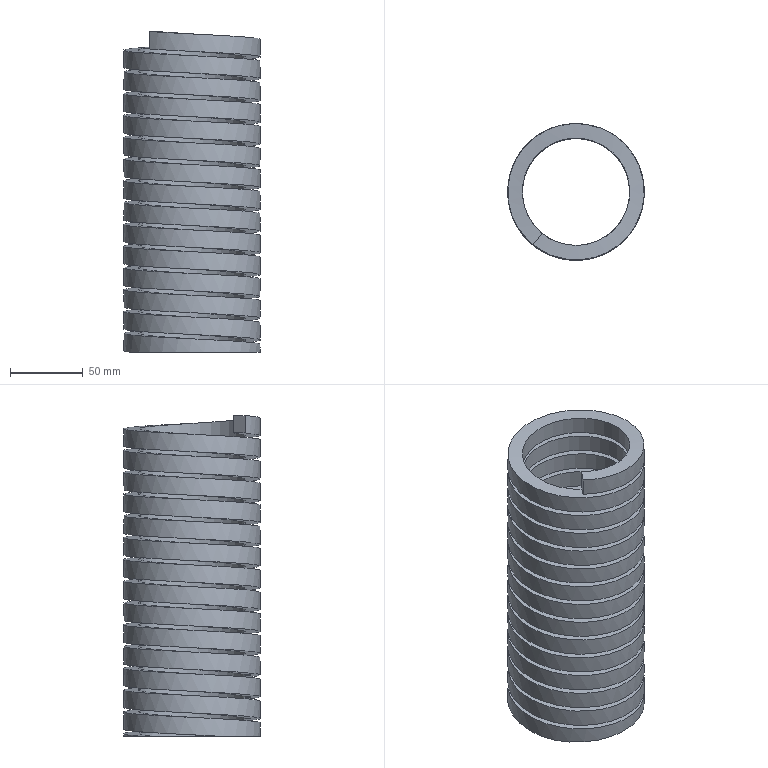Part | SolidWorks | features ICE 2, Helix 1, Sweep 1 | 1 solid | 22 faces | box 94 x 94 x 220.999 mm | volume 451222 mm3 | plane 14 | spline 8